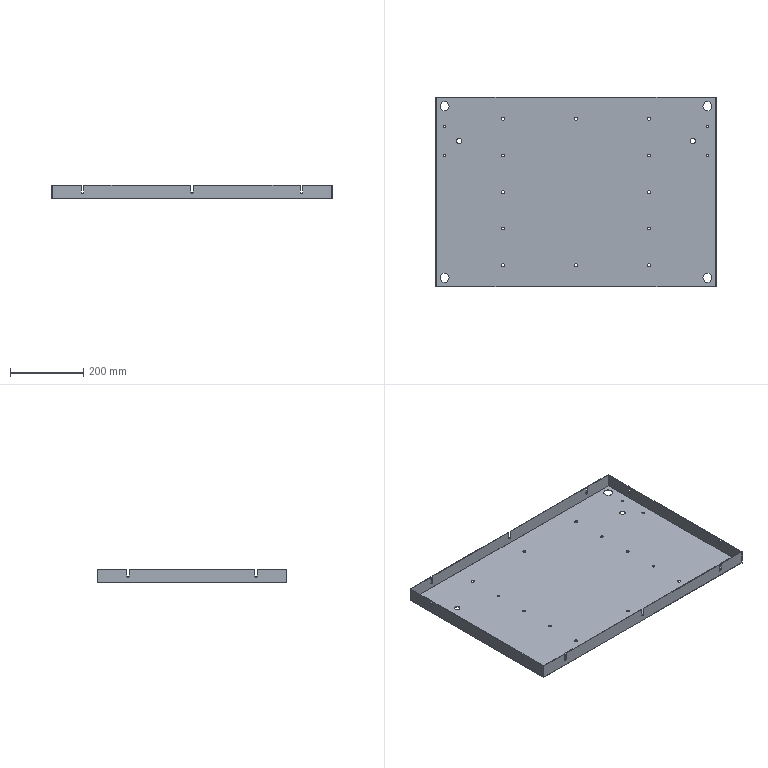Part | STEP file | Bottom seal plate | 1 solid | 98 faces | box 768 x 518 x 38 mm | volume 730452 mm3 | cylinder 58 | plane 40 | commonest cylinder face diameters 8.2 x16 7 x14 6.2 x8 6.5 x8 25 x8 15 x4